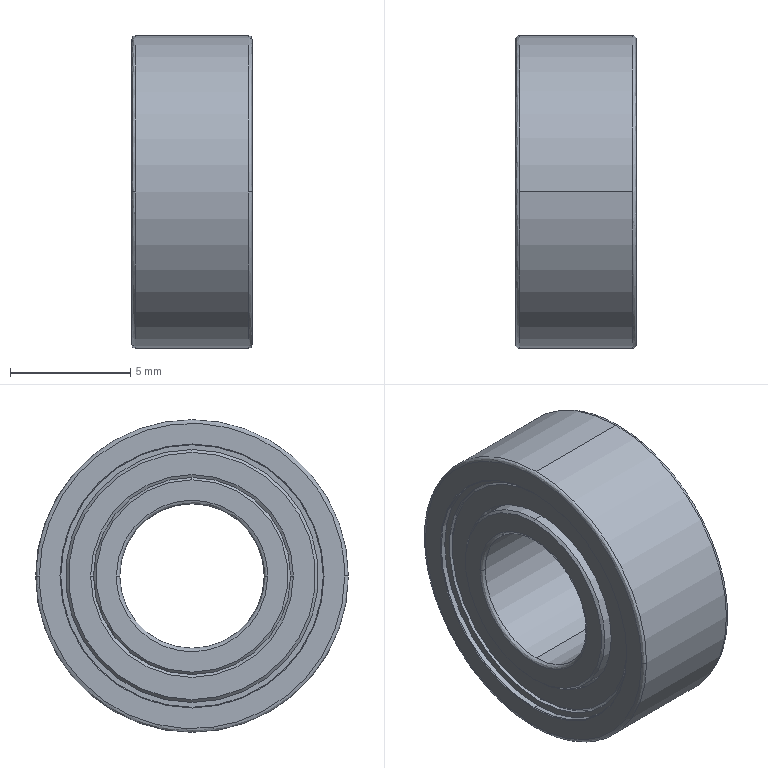Part | SolidWorks | features BaseBody 1 | 1 solid | 72 faces | box 5 x 13 x 13 mm | volume 402.825 mm3 | cylinder 24 | cone 24 | spline 12 | plane 12 | commonest cylinder face diameters 10.52 x8 8.2 x4 8.432 x4 10.92 x4 6 x2 13 x2